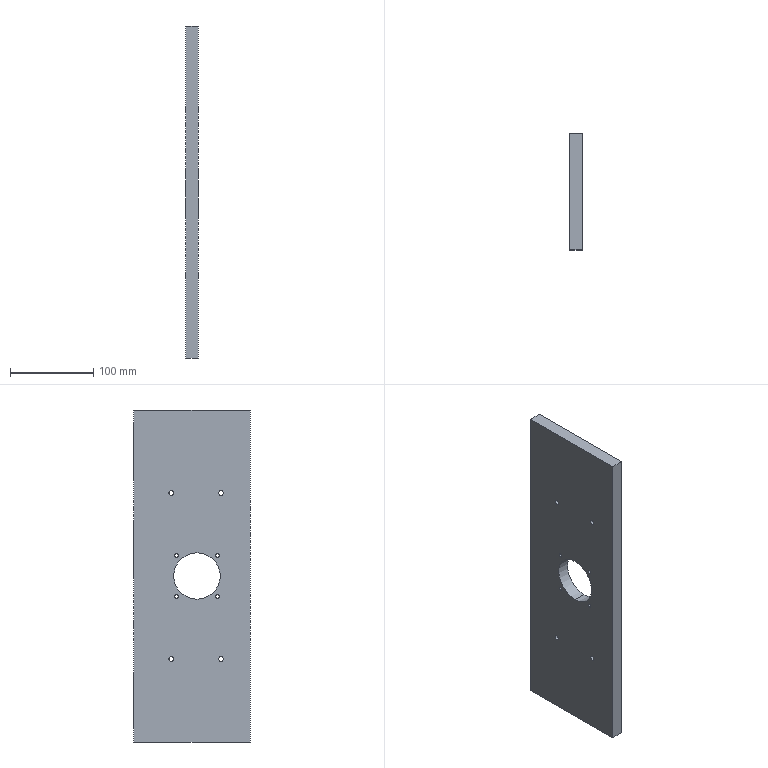Part | STEP file | 0244_216_Plate | 1 solid | 52 faces | box 15 x 140 x 400 mm | volume 795604 mm3 | cylinder 32 | cone 14 | plane 6 | commonest cylinder face diameters 6.8 x14 4.2 x8 5.5 x8 56 x2